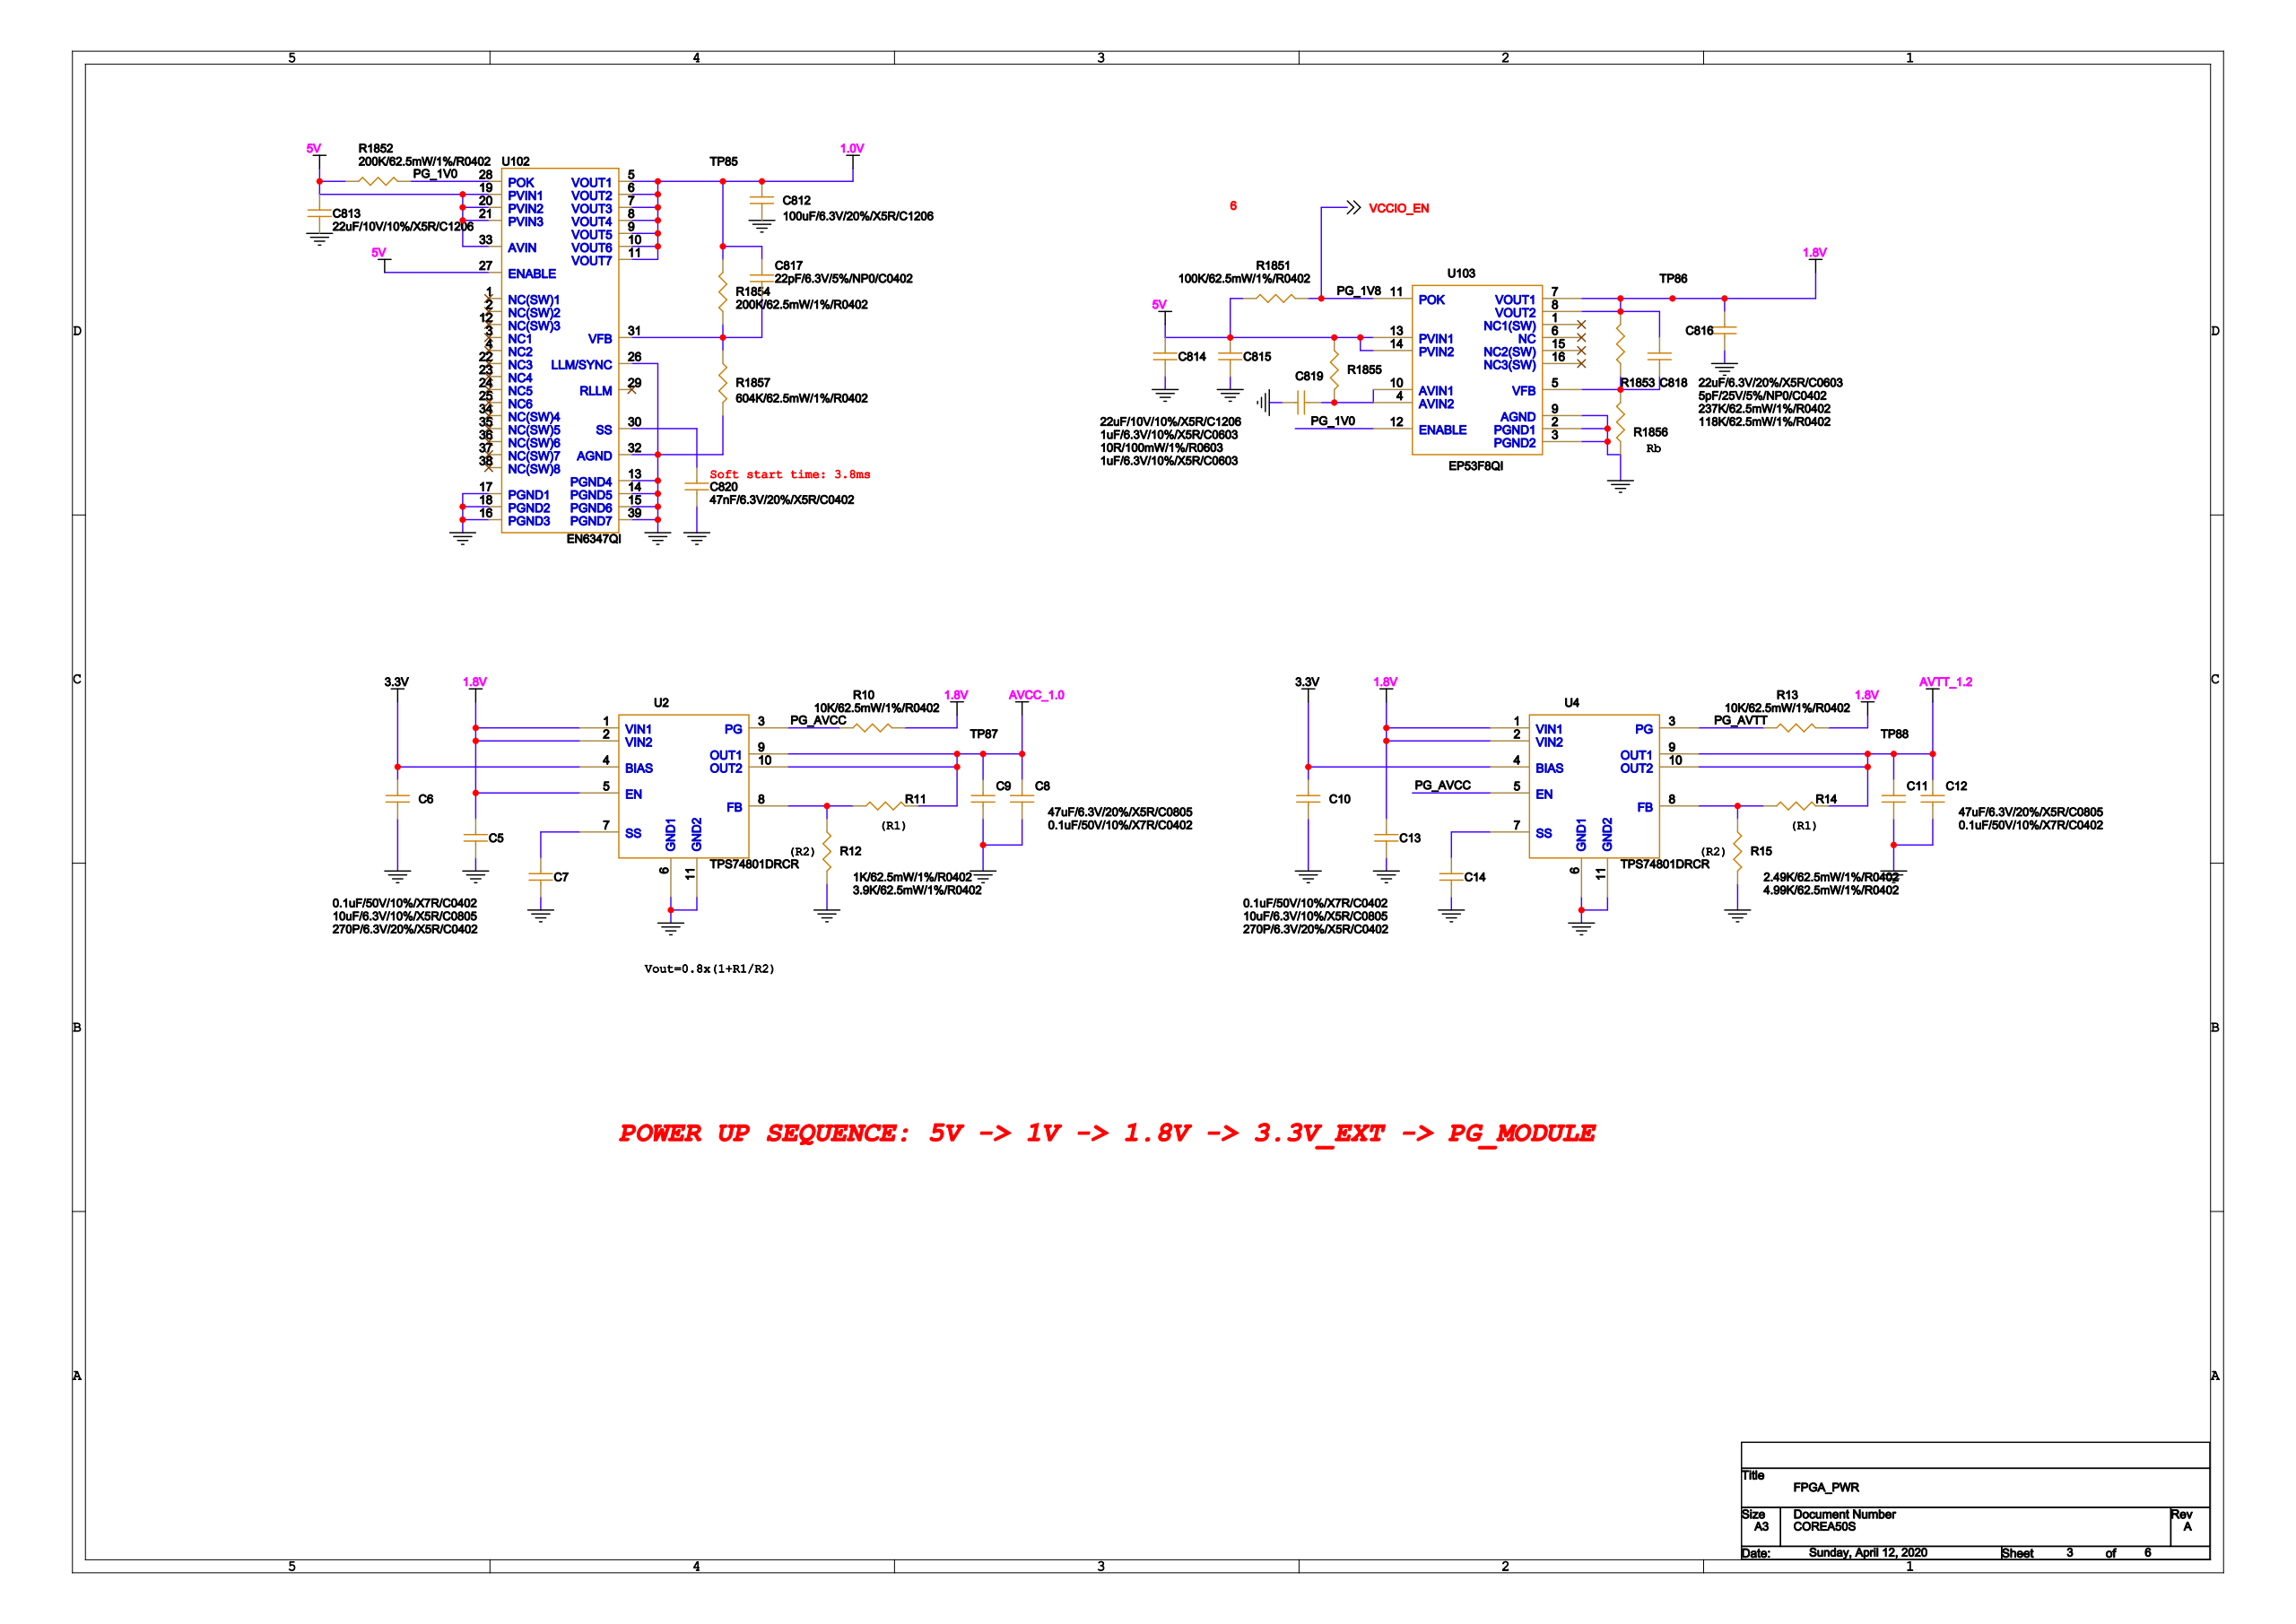Circuit board | Cadence Allegro | 202 parts | 354 nets | one sheet of the schematic
Parts on this sheet (reference | value | footprint):
C5 | 10uF/6.3V/10%/X5R/C0805 | 0805
C6 | 0.1uF/50V/10%/X7R/C0402 | 0402
C7 | 270P/6.3V/20%/X5R/C0402 | 0402
C8 | 0.1uF/50V/10%/X7R/C0402 | 0402
C9 | 47uF/6.3V/20%/X5R/C0805 | 0805
C10 | 0.1uF/50V/10%/X7R/C0402 | 0402
C11 | 47uF/6.3V/20%/X5R/C0805 | 0805
C12 | 0.1uF/50V/10%/X7R/C0402 | 0402
C13 | 10uF/6.3V/10%/X5R/C0805 | 0805
C14 | 270P/6.3V/20%/X5R/C0402 | 0402
C812 | 100uF/6.3V/20%/X5R/C1206 | T_1206
C813 | 22uF/10V/10%/X5R/C1206 | T_1206
C814 | 22uF/10V/10%/X5R/C1206 | T_1206
C815 | 1uF/6.3V/10%/X5R/C0603 | 0603
C816 | 22uF/6.3V/20%/X5R/C0603 | 0603
C817 | 22pF/6.3V/5%/NP0/C0402 | 0402
C818 | 5pF/25V/5%/NP0/C0402 | 0402
C819 | 1uF/6.3V/10%/X5R/C0603 | 0603
C820 | 47nF/6.3V/20%/X5R/C0402 | 0402
R10 | 10K/62.5mW/1%/R0402 | 0402
R11 | 1K/62.5mW/1%/R0402 | 0402
R12 | 3.9K/62.5mW/1%/R0402 | 0402
R13 | 10K/62.5mW/1%/R0402 | 0402
R14 | 2.49K/62.5mW/1%/R0402 | 0402
R15 | 4.99K/62.5mW/1%/R0402 | 0402
R1851 | 100K/62.5mW/1%/R0402 | 0402
R1852 | 200K/62.5mW/1%/R0402 | 0402
R1853 | 237K/62.5mW/1%/R0402 | 0402
R1854 | 200K/62.5mW/1%/R0402 | 0402
R1855 | 10R/100mW/1%/R0603 | 0603
R1856 | 118K/62.5mW/1%/R0402 | 0402
R1857 | 604K/62.5mW/1%/R0402 | 0402
TP85 | TEST POINT A | TEST_12MM
TP86 | TEST POINT A | TEST_12MM
TP87 | TEST POINT A | TEST_12MM
TP88 | TEST POINT A | TEST_12MM
U2 | TPS74801DRCR | VSON-10
U4 | TPS74801DRCR | VSON-10
U102 | EN6347QI | EN6347QI
U103 | EP53F8QI | QFN-16_3X3
Nets of these parts (net: part-pin ...):
GND: C5-2 C6-2 C7-2 C8-2 C9-2 C10-2 C11-2 C12-2 C13-2 C14-2 C812-2 C813-2 C814-2 C815-2 C816-2 C819-1 C820-2 R12-1 R15-1 R1856-2 R1857-1 U2-6 U2-11 U4-6 U4-11 U103-2 U103-3 U103-9 U102-13 U102-14 U102-15 U102-16 U102-17 U102-18 U102-26 U102-32 U102-39
3.3V: C6-1 C10-1 U2-4 U4-4
1.8V: C5-1 C13-1 C816-1 C818-1 R10-1 R13-1 R1853-1 TP86-1 U2-1 U2-2 U2-5 U4-1 U4-2 U103-7 U103-8
AVCC_1.0: C8-1 C9-1 R11-1 TP87-1 U2-9 U2-10
AVTT_1.2: C11-1 C12-1 R14-1 TP88-1 U4-9 U4-10
1.0V: C812-1 C817-1 R1854-1 TP85-1 U102-5 U102-6 U102-7 U102-8 U102-9 U102-10 U102-11
N26377193: R11-2 R12-2 U2-8
N26377809: C14-1 U4-7
N26375633: C7-1 U2-7
5V: C813-1 C814-1 C815-1 R1851-2 R1852-2 R1855-2 U103-13 U103-14 U102-19 U102-20 U102-21 U102-27 U102-33
VCCIO_EN: R1851-1 U103-11
PG_AVCC: R10-2 U2-3 U4-5
PG_AVTT: R13-2 U4-3
N26377917: R14-2 R15-2 U4-8
N26230881: C817-2 R1854-2 R1857-2 U102-31
N26230943: C820-1 U102-30
N26230875: C819-2 R1855-1 U103-4 U103-10
N26230857: C818-2 R1853-2 R1856-1 U103-5
PG_1V0: R1852-1 U103-12 U102-28